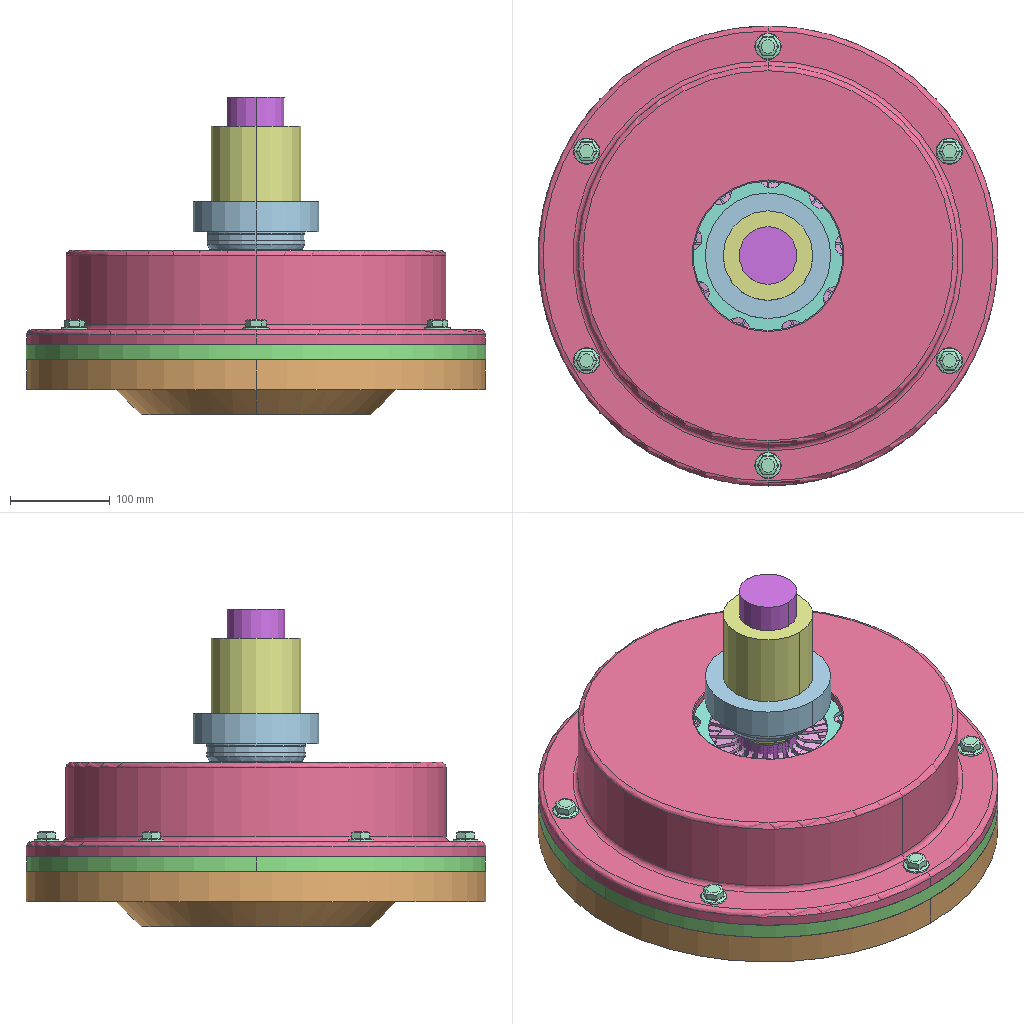Assembly | SolidWorks | 14 different items | 14 placed | box 461 x 461 x 318 mm
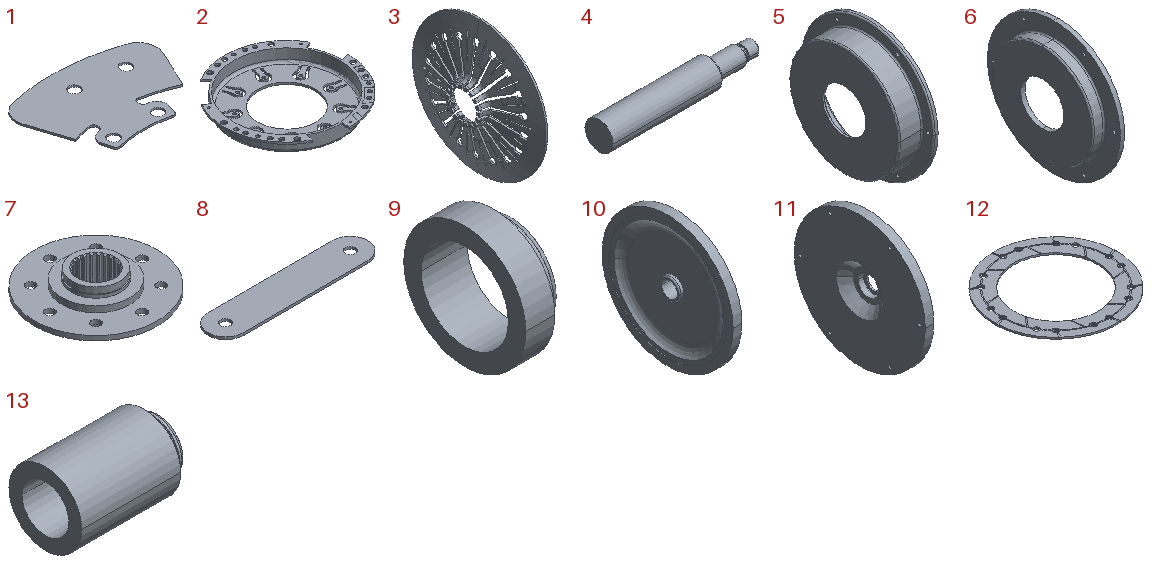Parts list (item | name | quantity | size | volume | features):
1 | - | x1 | 72.756 x 51.823 x 1 mm | 2634 mm3 | features Extrusion 1
2 | - | x1 | 260 x 260 x 30 mm | 210194 mm3 | features ICE 7, Fillet 2, Extrusion 1, Shell 1
3 | - | x1 | 30 x 220 x 220 mm | 90672 mm3 | features ICE 3, CirPattern 1, Revolution 1
4 | - | x1 | 317.85 x 58 x 58 mm | 690126 mm3 | features Revolution 1
5 | - | x1 | 94.6 x 461 x 461 mm | 3440559 mm3 | features Cut 1, Revolution 1
6 | - | x1 | 54.8 x 461 x 461 mm | 2855101 mm3 | features Cut 1, Revolution 1
7 | - | x1 | 80 x 80 x 26 mm | 24406 mm3 | features ICE 9, Extrusion 1, RevCut 1
8 | - | x1 | 64 x 14 x 1 mm | 828.805 mm3 | features Extrusion 1
9 | - | x1 | 47.5 x 126 x 126 mm | 203542 mm3 | features Revolution 1
10 | - | x1 | 40.5 x 315 x 315 mm | 1243951 mm3 | features Revolution 1
11 | - | x1 | 55 x 461 x 461 mm | 5743075 mm3 | features Cut 1, Revolution 1
12 | - | x1 | 220 x 220 x 3 mm | 57628 mm3 | features ICE 3, Extrusion 1
13 | - | x1 | 139.56 x 90 x 90 mm | 471413 mm3 | features Revolution 1
14 | hex flange bolts-heavy grade b gb | x1 | - | - | -
Mates (type | each side: item.copy, entity, surface, feature):
Concentric | 12.1 face cylinder Boss-Extrude1 | 7.1 face cylinder Boss-Extrude1
Concentric | 1.1 face cylinder Boss-Extrude2 | 12.1 face cylinder Cut-Extrude2
Coincident | 1.1 face plane Boss-Extrude2 | 12.1 face plane Boss-Extrude1
Coincident | 1.1 face plane Boss-Extrude2 | 7.1 face plane Boss-Extrude1
Concentric | 13.1 face cylinder Revolve1 | 4.1 face cylinder Revolve1
Concentric | 9.1 face cylinder Revolve1 | 13.1 face cylinder Revolve1
Coincident | 11.1 face plane Revolve1 | 4.1 face plane Revolve1
Concentric | 11.1 face cylinder Revolve1 | 4.1 face cylinder Revolve1
Concentric | 7.1 face cylinder Boss-Extrude4 | 4.1 face cylinder Revolve1
Coincident | 1.1 face plane Boss-Extrude2 | 11.1 face plane Revolve1
Coincident | 11.1 face plane Revolve1 | 10.1 face plane Revolve1
Concentric | 10.1 face cylinder Revolve1 | 4.1 face cylinder Revolve1
Coincident | 11.1 face plane Revolve1 | 6.1 face plane Revolve1
Concentric | 6.1 face cylinder Revolve1 | 4.1 face cylinder Revolve1
Coincident | 6.1 face plane Revolve1 | 5.1 face plane Revolve2
Concentric | 5.1 face cylinder Revolve2 | 4.1 face cylinder Revolve1
Concentric | 3.1 face cylinder Cut-Extrude5 | 4.1 face cylinder Revolve1
Concentric | 2.1 face cylinder Boss-Extrude1 | 4.1 face cylinder Revolve1
Coincident | 2.1 face plane Boss-Extrude1 | 5.1 face plane Revolve2
Coincident | 3.1 face plane Revolve1 | 2.1 face plane Shell1
Coincident | 2.1 face plane Boss-Extrude1 | 13.1 face plane Revolve1